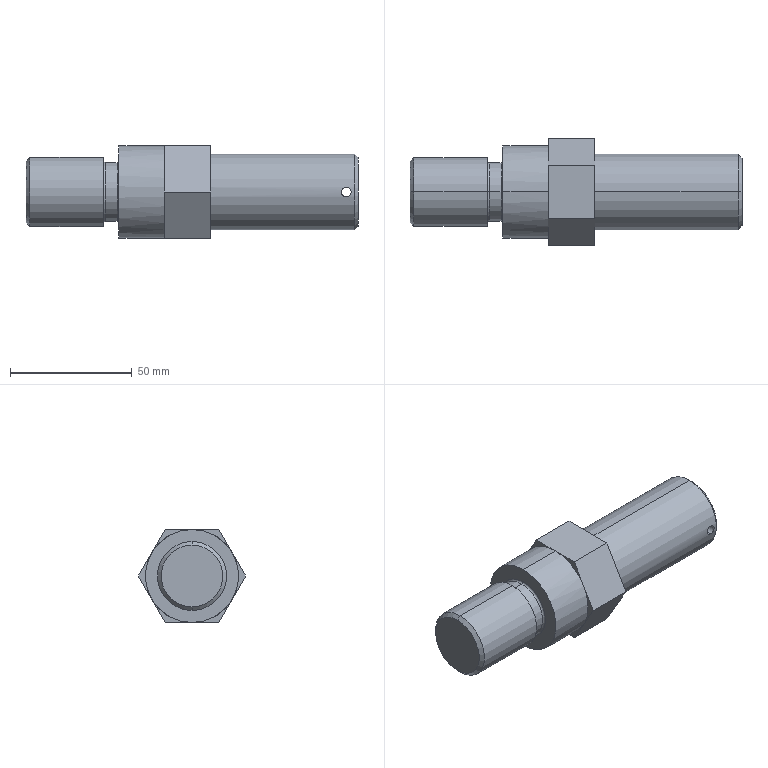Part | SolidWorks | features ICE 2, Chamfer 1, Fillet 1, Revolution 1 | 1 solid | 35 faces | box 136.144 x 43.994 x 38.1 mm | volume 113370 mm3 | plane 17 | cylinder 10 | torus 4 | cone 4 | commonest cylinder face diameters 3.969 x2 24.13 x2 28.321 x2 31.115 x2 38.1 x2
STEP:
#1=CARTESIAN_POINT('',(131.318,-15.43,-1.984));
#2=VERTEX_POINT('',#1);
#3=CARTESIAN_POINT('',(131.318,-15.43,1.984));
#4=VERTEX_POINT('',#3);
#5=CARTESIAN_POINT('',(131.318,-15.43,-1.984));
#6=CARTESIAN_POINT('',(131.059,-15.43,-1.984));
#7=CARTESIAN_POINT('',(130.798,-15.437,-1.932));
#8=CARTESIAN_POINT('',(130.32,-15.461,-1.734));
#9=CARTESIAN_POINT('',(130.099,-15.477,-1.587));
#10=CARTESIAN_POINT('',(129.824,-15.502,-1.313));
#11=CARTESIAN_POINT('',(129.74,-15.511,-1.211));
#12=CARTESIAN_POINT('',(129.596,-15.526,-0.9954));
#13=CARTESIAN_POINT('',(129.535,-15.533,-0.8815));
#14=CARTESIAN_POINT('',(129.436,-15.545,-0.6413));
#15=CARTESIAN_POINT('',(129.397,-15.549,-0.5153));
#16=CARTESIAN_POINT('',(129.347,-15.556,-0.2617));
#17=CARTESIAN_POINT('',(129.334,-15.557,-0.1326));
#18=CARTESIAN_POINT('',(129.334,-15.558,0.1298));
#19=CARTESIAN_POINT('',(129.346,-15.556,0.2588));
#20=CARTESIAN_POINT('',(129.397,-15.55,0.5126));
#21=CARTESIAN_POINT('',(129.435,-15.545,0.6388));
#22=CARTESIAN_POINT('',(129.534,-15.533,0.879));
#23=CARTESIAN_POINT('',(129.595,-15.526,0.993));
#24=CARTESIAN_POINT('',(129.739,-15.511,1.209));
#25=CARTESIAN_POINT('',(129.823,-15.502,1.311));
#26=CARTESIAN_POINT('',(130.097,-15.478,1.585));
#27=CARTESIAN_POINT('',(130.318,-15.461,1.733));
#28=CARTESIAN_POINT('',(130.795,-15.437,1.932));
#29=CARTESIAN_POINT('',(131.056,-15.43,1.984));
#30=CARTESIAN_POINT('',(131.318,-15.43,1.984));
#31=B_SPLINE_CURVE_WITH_KNOTS('',3,(#5,#6,#7,#8,#9,#10,#11,#12,#13,#14,#15,#16,#17,#18,#19,#20,#21,#22,#23,#24,#25,#26,#27,#28,#29,#30),.UNSPECIFIED.,.F.,.F.,(4,2,2,2,2,2,2,2,2,2,2,2,4),(0.00621,0.006986,0.007763,0.008151,0.008539,0.008927,0.009315,0.009703,0.01009,0.01048,0.01087,0.01164,0.01242),.UNSPECIFIED.);
#32=EDGE_CURVE('',#2,#4,#31,.T.);
#33=ORIENTED_EDGE('',*,*,#32,.F.);
#34=CARTESIAN_POINT('',(131.318,15.43,-1.984));
#35=VERTEX_POINT('',#34);
#36=CARTESIAN_POINT('',(131.318,-25.,-1.984));
#37=DIRECTION('',(0.,1.,0.));
#38=VECTOR('',#37,1000.);
#39=LINE('',#36,#38);
#40=EDGE_CURVE('',#2,#35,#39,.T.);
#41=ORIENTED_EDGE('',*,*,#40,.T.);
#42=CARTESIAN_POINT('',(131.318,15.43,1.984));
#43=VERTEX_POINT('',#42);
#44=CARTESIAN_POINT('',(131.318,15.43,1.984));
#45=CARTESIAN_POINT('',(131.187,15.43,1.984));
#46=CARTESIAN_POINT('',(131.058,15.432,1.971));
#47=CARTESIAN_POINT('',(130.804,15.438,1.921));
#48=CARTESIAN_POINT('',(130.678,15.443,1.883));
#49=CARTESIAN_POINT('',(130.438,15.455,1.783));
#50=CARTESIAN_POINT('',(130.324,15.462,1.722));
#51=CARTESIAN_POINT('',(130.108,15.477,1.578));
#52=CARTESIAN_POINT('',(130.006,15.486,1.494));
#53=CARTESIAN_POINT('',(129.732,15.511,1.22));
#54=CARTESIAN_POINT('',(129.584,15.527,0.9987));
#55=CARTESIAN_POINT('',(129.386,15.551,0.5212));
#56=CARTESIAN_POINT('',(129.334,15.557,0.2599));
#57=CARTESIAN_POINT('',(129.334,15.558,-0.1288));
#58=CARTESIAN_POINT('',(129.347,15.556,-0.2605));
#59=CARTESIAN_POINT('',(129.397,15.549,-0.5151));
#60=CARTESIAN_POINT('',(129.435,15.545,-0.6389));
#61=CARTESIAN_POINT('',(129.534,15.533,-0.8793));
#62=CARTESIAN_POINT('',(129.596,15.526,-0.9953));
#63=CARTESIAN_POINT('',(129.74,15.511,-1.21));
#64=CARTESIAN_POINT('',(129.822,15.502,-1.31));
#65=CARTESIAN_POINT('',(130.007,15.486,-1.496));
#66=CARTESIAN_POINT('',(130.107,15.477,-1.578));
#67=CARTESIAN_POINT('',(130.322,15.462,-1.721));
#68=CARTESIAN_POINT('',(130.438,15.455,-1.783));
#69=CARTESIAN_POINT('',(130.679,15.443,-1.883));
#70=CARTESIAN_POINT('',(130.802,15.439,-1.921));
#71=CARTESIAN_POINT('',(131.057,15.432,-1.971));
#72=CARTESIAN_POINT('',(131.188,15.43,-1.984));
#73=CARTESIAN_POINT('',(131.318,15.43,-1.984));
#74=B_SPLINE_CURVE_WITH_KNOTS('',3,(#44,#45,#46,#47,#48,#49,#50,#51,#52,#53,#54,#55,#56,#57,#58,#59,#60,#61,#62,#63,#64,#65,#66,#67,#68,#69,#70,#71,#72,#73),.UNSPECIFIED.,.F.,.F.,(4,2,2,2,2,2,2,2,2,2,2,2,2,2,4),(0.,0.0003881,0.0007763,0.001164,0.001553,0.002329,0.003105,0.003493,0.003881,0.00427,0.004658,0.005046,0.005434,0.005822,0.00621),.UNSPECIFIED.);
#75=EDGE_CURVE('',#43,#35,#74,.T.);
#76=ORIENTED_EDGE('',*,*,#75,.F.);
#77=CARTESIAN_POINT('',(131.318,-25.,1.984));
#78=DIRECTION('',(0.,1.,0.));
#79=VECTOR('',#78,1000.);
#80=LINE('',#77,#79);
#81=EDGE_CURVE('',#4,#43,#80,.T.);
#82=ORIENTED_EDGE('',*,*,#81,.F.);
#83=EDGE_LOOP('',(#33,#41,#76,#82));
#84=FACE_OUTER_BOUND('',#83,.T.);
#85=CARTESIAN_POINT('',(131.318,-25.,0.));
#86=DIRECTION('',(0.,1.,0.));
#87=DIRECTION('',(0.,0.,1.));
#88=AXIS2_PLACEMENT_3D('',#85,#86,#87);
#89=CYLINDRICAL_SURFACE('',#88,1.984);
#90=ADVANCED_FACE('',(#84),#89,.F.);
#91=CARTESIAN_POINT('',(38.1,0.,12.827));
#92=VERTEX_POINT('',#91);
#93=CARTESIAN_POINT('',(38.1,0.,-12.827));
#94=VERTEX_POINT('',#93);
#95=CARTESIAN_POINT('',(38.1,0.,0.));
#96=DIRECTION('',(1.,0.,0.));
#97=DIRECTION('',(0.,0.,-1.));
#98=AXIS2_PLACEMENT_3D('',#95,#96,#97);
#99=CIRCLE('',#98,12.827);
#100=EDGE_CURVE('',#92,#94,#99,.T.);
#101=ORIENTED_EDGE('',*,*,#100,.F.);
#102=CARTESIAN_POINT('',(37.338,0.,12.065));
#103=VERTEX_POINT('',#102);
#104=CARTESIAN_POINT('',(37.338,0.,12.827));
#105=DIRECTION('',(0.,1.,0.));
#106=DIRECTION('',(0.,0.,1.));
#107=AXIS2_PLACEMENT_3D('',#104,#105,#106);
#108=CIRCLE('',#107,0.762);
#109=EDGE_CURVE('',#92,#103,#108,.T.);
#110=ORIENTED_EDGE('',*,*,#109,.T.);
#111=CARTESIAN_POINT('',(37.338,0.,-12.065));
#112=VERTEX_POINT('',#111);
#113=CARTESIAN_POINT('',(37.338,0.,0.));
#114=DIRECTION('',(-1.,0.,0.));
#115=DIRECTION('',(0.,0.,-1.));
#116=AXIS2_PLACEMENT_3D('',#113,#114,#115);
#117=CIRCLE('',#116,12.065);
#118=EDGE_CURVE('',#112,#103,#117,.T.);
#119=ORIENTED_EDGE('',*,*,#118,.F.);
#120=CARTESIAN_POINT('',(37.338,0.,-12.827));
#121=DIRECTION('',(0.,-1.,0.));
#122=DIRECTION('',(0.,0.,-1.));
#123=AXIS2_PLACEMENT_3D('',#120,#121,#122);
#124=CIRCLE('',#123,0.762);
#125=EDGE_CURVE('',#94,#112,#124,.T.);
#126=ORIENTED_EDGE('',*,*,#125,.F.);
#127=EDGE_LOOP('',(#101,#110,#119,#126));
#128=FACE_OUTER_BOUND('',#127,.T.);
#129=CARTESIAN_POINT('',(37.338,0.,0.));
#130=DIRECTION('',(1.,0.,0.));
#131=DIRECTION('',(0.,0.,-1.));
#132=AXIS2_PLACEMENT_3D('',#129,#130,#131);
#133=TOROIDAL_SURFACE('',#132,12.827,0.762);
#134=ADVANCED_FACE('',(#128),#133,.F.);
#135=CARTESIAN_POINT('',(31.75,0.,-12.827));
#136=VERTEX_POINT('',#135);
#137=CARTESIAN_POINT('',(31.75,0.,12.827));
#138=VERTEX_POINT('',#137);
#139=CARTESIAN_POINT('',(31.75,0.,0.));
#140=DIRECTION('',(-1.,0.,0.));
#141=DIRECTION('',(0.,0.,1.));
#142=AXIS2_PLACEMENT_3D('',#139,#140,#141);
#143=CIRCLE('',#142,12.827);
#144=EDGE_CURVE('',#136,#138,#143,.T.);
#145=ORIENTED_EDGE('',*,*,#144,.F.);
#146=CARTESIAN_POINT('',(32.512,0.,-12.065));
#147=VERTEX_POINT('',#146);
#148=CARTESIAN_POINT('',(32.512,0.,-12.827));
#149=DIRECTION('',(0.,1.,0.));
#150=DIRECTION('',(0.,0.,1.));
#151=AXIS2_PLACEMENT_3D('',#148,#149,#150);
#152=CIRCLE('',#151,0.762);
#153=EDGE_CURVE('',#136,#147,#152,.T.);
#154=ORIENTED_EDGE('',*,*,#153,.T.);
#155=CARTESIAN_POINT('',(32.512,0.,12.065));
#156=VERTEX_POINT('',#155);
#157=CARTESIAN_POINT('',(32.512,0.,0.));
#158=DIRECTION('',(1.,0.,0.));
#159=DIRECTION('',(0.,0.,1.));
#160=AXIS2_PLACEMENT_3D('',#157,#158,#159);
#161=CIRCLE('',#160,12.065);
#162=EDGE_CURVE('',#156,#147,#161,.T.);
#163=ORIENTED_EDGE('',*,*,#162,.F.);
#164=CARTESIAN_POINT('',(32.512,0.,12.827));
#165=DIRECTION('',(0.,-1.,0.));
#166=DIRECTION('',(0.,0.,-1.));
#167=AXIS2_PLACEMENT_3D('',#164,#165,#166);
#168=CIRCLE('',#167,0.762);
#169=EDGE_CURVE('',#138,#156,#168,.T.);
#170=ORIENTED_EDGE('',*,*,#169,.F.);
#171=EDGE_LOOP('',(#145,#154,#163,#170));
#172=FACE_OUTER_BOUND('',#171,.T.);
#173=CARTESIAN_POINT('',(32.512,0.,0.));
#174=DIRECTION('',(-1.,0.,0.));
#175=DIRECTION('',(0.,0.,1.));
#176=AXIS2_PLACEMENT_3D('',#173,#174,#175);
#177=TOROIDAL_SURFACE('',#176,12.827,0.762);
#178=ADVANCED_FACE('',(#172),#177,.F.);
#179=ORIENTED_EDGE('',*,*,#75,.T.);
#180=CARTESIAN_POINT('',(131.318,15.43,-1.984));
#181=CARTESIAN_POINT('',(131.577,15.43,-1.984));
#182=CARTESIAN_POINT('',(131.838,15.437,-1.932));
#183=CARTESIAN_POINT('',(132.316,15.461,-1.734));
#184=CARTESIAN_POINT('',(132.537,15.477,-1.587));
#185=CARTESIAN_POINT('',(132.812,15.502,-1.313));
#186=CARTESIAN_POINT('',(132.896,15.511,-1.211));
#187=CARTESIAN_POINT('',(133.04,15.526,-0.9954));
#188=CARTESIAN_POINT('',(133.101,15.533,-0.8815));
#189=CARTESIAN_POINT('',(133.2,15.545,-0.6413));
#190=CARTESIAN_POINT('',(133.239,15.549,-0.5153));
#191=CARTESIAN_POINT('',(133.289,15.556,-0.2617));
#192=CARTESIAN_POINT('',(133.302,15.557,-0.1326));
#193=CARTESIAN_POINT('',(133.302,15.558,0.1298));
#194=CARTESIAN_POINT('',(133.29,15.556,0.2588));
#195=CARTESIAN_POINT('',(133.239,15.55,0.5126));
#196=CARTESIAN_POINT('',(133.201,15.545,0.6388));
#197=CARTESIAN_POINT('',(133.102,15.533,0.879));
#198=CARTESIAN_POINT('',(133.041,15.526,0.993));
#199=CARTESIAN_POINT('',(132.897,15.511,1.209));
#200=CARTESIAN_POINT('',(132.813,15.502,1.311));
#201=CARTESIAN_POINT('',(132.539,15.478,1.585));
#202=CARTESIAN_POINT('',(132.318,15.461,1.733));
#203=CARTESIAN_POINT('',(131.841,15.437,1.932));
#204=CARTESIAN_POINT('',(131.58,15.43,1.984));
#205=CARTESIAN_POINT('',(131.318,15.43,1.984));
#206=B_SPLINE_CURVE_WITH_KNOTS('',3,(#180,#181,#182,#183,#184,#185,#186,#187,#188,#189,#190,#191,#192,#193,#194,#195,#196,#197,#198,#199,#200,#201,#202,#203,#204,#205),.UNSPECIFIED.,.F.,.F.,(4,2,2,2,2,2,2,2,2,2,2,2,4),(0.00621,0.006986,0.007763,0.008151,0.008539,0.008927,0.009315,0.009703,0.01009,0.01048,0.01087,0.01164,0.01242),.UNSPECIFIED.);
#207=EDGE_CURVE('',#35,#43,#206,.T.);
#208=ORIENTED_EDGE('',*,*,#207,.T.);
#209=EDGE_LOOP('',(#179,#208));
#210=FACE_BOUND('',#209,.T.);
#211=CARTESIAN_POINT('',(134.62,0.,15.557));
#212=VERTEX_POINT('',#211);
#213=CARTESIAN_POINT('',(134.62,0.,-15.557));
#214=VERTEX_POINT('',#213);
#215=CARTESIAN_POINT('',(134.62,0.,0.));
#216=DIRECTION('',(-1.,0.,0.));
#217=DIRECTION('',(0.,0.,1.));
#218=AXIS2_PLACEMENT_3D('',#215,#216,#217);
#219=CIRCLE('',#218,15.557);
#220=EDGE_CURVE('',#212,#214,#219,.T.);
#221=ORIENTED_EDGE('',*,*,#220,.T.);
#222=CARTESIAN_POINT('',(75.692,0.,-15.557));
#223=VERTEX_POINT('',#222);
#224=CARTESIAN_POINT('',(0.,0.,-15.557));
#225=DIRECTION('',(-1.,0.,0.));
#226=VECTOR('',#225,1000.);
#227=LINE('',#224,#226);
#228=EDGE_CURVE('',#214,#223,#227,.T.);
#229=ORIENTED_EDGE('',*,*,#228,.T.);
#230=CARTESIAN_POINT('',(75.692,0.,15.557));
#231=VERTEX_POINT('',#230);
#232=CARTESIAN_POINT('',(75.692,0.,0.));
#233=DIRECTION('',(-1.,0.,0.));
#234=DIRECTION('',(0.,0.,1.));
#235=AXIS2_PLACEMENT_3D('',#232,#233,#234);
#236=CIRCLE('',#235,15.557);
#237=EDGE_CURVE('',#231,#223,#236,.T.);
#238=ORIENTED_EDGE('',*,*,#237,.F.);
#239=CARTESIAN_POINT('',(0.,0.,15.557));
#240=DIRECTION('',(-1.,0.,0.));
#241=VECTOR('',#240,1000.);
#242=LINE('',#239,#241);
#243=EDGE_CURVE('',#212,#231,#242,.T.);
#244=ORIENTED_EDGE('',*,*,#243,.F.);
#245=EDGE_LOOP('',(#221,#229,#238,#244));
#246=FACE_OUTER_BOUND('',#245,.T.);
#247=CARTESIAN_POINT('',(0.,0.,0.));
#248=DIRECTION('',(-1.,0.,0.));
#249=DIRECTION('',(0.,0.,1.));
#250=AXIS2_PLACEMENT_3D('',#247,#248,#249);
#251=CYLINDRICAL_SURFACE('',#250,15.557);
#252=ADVANCED_FACE('',(#210,#246),#251,.T.);
#253=CARTESIAN_POINT('',(136.144,0.,-14.034));
#254=VERTEX_POINT('',#253);
#255=CARTESIAN_POINT('',(136.144,0.,14.034));
#256=VERTEX_POINT('',#255);
#257=CARTESIAN_POINT('',(136.144,0.,0.));
#258=DIRECTION('',(1.,0.,0.));
#259=DIRECTION('',(0.,0.,1.));
#260=AXIS2_PLACEMENT_3D('',#257,#258,#259);
#261=CIRCLE('',#260,14.034);
#262=EDGE_CURVE('',#254,#256,#261,.T.);
#263=ORIENTED_EDGE('',*,*,#262,.F.);
#264=CARTESIAN_POINT('',(134.62,0.,-15.557));
#265=DIRECTION('',(-0.7071,0.,-0.7071));
#266=VECTOR('',#265,1000.);
#267=LINE('',#264,#266);
#268=EDGE_CURVE('',#254,#214,#267,.T.);
#269=ORIENTED_EDGE('',*,*,#268,.T.);
#270=ORIENTED_EDGE('',*,*,#220,.F.);
#271=CARTESIAN_POINT('',(134.62,0.,15.557));
#272=DIRECTION('',(-0.7071,0.,0.7071));
#273=VECTOR('',#272,1000.);
#274=LINE('',#271,#273);
#275=EDGE_CURVE('',#256,#212,#274,.T.);
#276=ORIENTED_EDGE('',*,*,#275,.F.);
#277=EDGE_LOOP('',(#263,#269,#270,#276));
#278=FACE_OUTER_BOUND('',#277,.T.);
#279=CARTESIAN_POINT('',(134.62,0.,0.));
#280=DIRECTION('',(-1.,0.,0.));
#281=DIRECTION('',(0.,0.,1.));
#282=AXIS2_PLACEMENT_3D('',#279,#280,#281);
#283=CONICAL_SURFACE('',#282,15.557,0.7854);
#284=ADVANCED_FACE('',(#278),#283,.T.);
#285=CARTESIAN_POINT('',(0.,0.,12.636));
#286=VERTEX_POINT('',#285);
#287=CARTESIAN_POINT('',(0.,0.,-12.636));
#288=VERTEX_POINT('',#287);
#289=CARTESIAN_POINT('',(0.,0.,0.));
#290=DIRECTION('',(-1.,0.,0.));
#291=DIRECTION('',(0.,0.,-1.));
#292=AXIS2_PLACEMENT_3D('',#289,#290,#291);
#293=CIRCLE('',#292,12.636);
#294=EDGE_CURVE('',#286,#288,#293,.T.);
#295=ORIENTED_EDGE('',*,*,#294,.F.);
#296=CARTESIAN_POINT('',(1.524,0.,14.161));
#297=VERTEX_POINT('',#296);
#298=CARTESIAN_POINT('',(0.,0.,12.636));
#299=DIRECTION('',(0.7071,0.,0.7071));
#300=VECTOR('',#299,1000.);
#301=LINE('',#298,#300);
#302=EDGE_CURVE('',#286,#297,#301,.T.);
#303=ORIENTED_EDGE('',*,*,#302,.T.);
#304=CARTESIAN_POINT('',(1.524,0.,-14.161));
#305=VERTEX_POINT('',#304);
#306=CARTESIAN_POINT('',(1.524,0.,0.));
#307=DIRECTION('',(1.,0.,0.));
#308=DIRECTION('',(0.,0.,-1.));
#309=AXIS2_PLACEMENT_3D('',#306,#307,#308);
#310=CIRCLE('',#309,14.161);
#311=EDGE_CURVE('',#305,#297,#310,.T.);
#312=ORIENTED_EDGE('',*,*,#311,.F.);
#313=CARTESIAN_POINT('',(0.,0.,-12.636));
#314=DIRECTION('',(0.7071,0.,-0.7071));
#315=VECTOR('',#314,1000.);
#316=LINE('',#313,#315);
#317=EDGE_CURVE('',#288,#305,#316,.T.);
#318=ORIENTED_EDGE('',*,*,#317,.F.);
#319=EDGE_LOOP('',(#295,#303,#312,#318));
#320=FACE_OUTER_BOUND('',#319,.T.);
#321=CARTESIAN_POINT('',(0.,0.,0.));
#322=DIRECTION('',(1.,0.,0.));
#323=DIRECTION('',(0.,0.,-1.));
#324=AXIS2_PLACEMENT_3D('',#321,#322,#323);
#325=CONICAL_SURFACE('',#324,12.636,0.7854);
#326=ADVANCED_FACE('',(#320),#325,.T.);
#327=CARTESIAN_POINT('',(37.338,0.,0.));
#328=DIRECTION('',(-1.,0.,0.));
#329=DIRECTION('',(0.,0.,-1.));
#330=AXIS2_PLACEMENT_3D('',#327,#328,#329);
#331=CIRCLE('',#330,12.065);
#332=EDGE_CURVE('',#103,#112,#331,.T.);
#333=ORIENTED_EDGE('',*,*,#332,.T.);
#334=CARTESIAN_POINT('',(0.,0.,-12.065));
#335=DIRECTION('',(-1.,0.,0.));
#336=VECTOR('',#335,1000.);
#337=LINE('',#334,#336);
#338=EDGE_CURVE('',#112,#147,#337,.T.);
#339=ORIENTED_EDGE('',*,*,#338,.T.);
#340=CARTESIAN_POINT('',(32.512,0.,0.));
#341=DIRECTION('',(1.,0.,0.));
#342=DIRECTION('',(0.,0.,1.));
#343=AXIS2_PLACEMENT_3D('',#340,#341,#342);
#344=CIRCLE('',#343,12.065);
#345=EDGE_CURVE('',#147,#156,#344,.T.);
#346=ORIENTED_EDGE('',*,*,#345,.T.);
#347=CARTESIAN_POINT('',(0.,0.,12.065));
#348=DIRECTION('',(-1.,0.,0.));
#349=VECTOR('',#348,1000.);
#350=LINE('',#347,#349);
#351=EDGE_CURVE('',#103,#156,#350,.T.);
#352=ORIENTED_EDGE('',*,*,#351,.F.);
#353=EDGE_LOOP('',(#333,#339,#346,#352));
#354=FACE_OUTER_BOUND('',#353,.T.);
#355=CARTESIAN_POINT('',(0.,0.,0.));
#356=DIRECTION('',(-1.,0.,0.));
#357=DIRECTION('',(0.,0.,1.));
#358=AXIS2_PLACEMENT_3D('',#355,#356,#357);
#359=CYLINDRICAL_SURFACE('',#358,12.065);
#360=ADVANCED_FACE('',(#354),#359,.T.);
#361=CARTESIAN_POINT('',(31.75,0.,14.161));
#362=VERTEX_POINT('',#361);
#363=CARTESIAN_POINT('',(31.75,0.,-14.161));
#364=VERTEX_POINT('',#363);
#365=CARTESIAN_POINT('',(31.75,0.,0.));
#366=DIRECTION('',(-1.,0.,0.));
#367=DIRECTION('',(0.,0.,1.));
#368=AXIS2_PLACEMENT_3D('',#365,#366,#367);
#369=CIRCLE('',#368,14.161);
#370=EDGE_CURVE('',#362,#364,#369,.T.);
#371=ORIENTED_EDGE('',*,*,#370,.T.);
#372=CARTESIAN_POINT('',(0.,0.,-14.161));
#373=DIRECTION('',(-1.,0.,0.));
#374=VECTOR('',#373,1000.);
#375=LINE('',#372,#374);
#376=EDGE_CURVE('',#364,#305,#375,.T.);
#377=ORIENTED_EDGE('',*,*,#376,.T.);
#378=ORIENTED_EDGE('',*,*,#311,.T.);
#379=CARTESIAN_POINT('',(0.,0.,14.161));
#380=DIRECTION('',(-1.,0.,0.));
#381=VECTOR('',#380,1000.);
#382=LINE('',#379,#381);
#383=EDGE_CURVE('',#362,#297,#382,.T.);
#384=ORIENTED_EDGE('',*,*,#383,.F.);
#385=EDGE_LOOP('',(#371,#377,#378,#384));
#386=FACE_OUTER_BOUND('',#385,.T.);
#387=CARTESIAN_POINT('',(0.,0.,0.));
#388=DIRECTION('',(-1.,0.,0.));
#389=DIRECTION('',(0.,0.,1.));
#390=AXIS2_PLACEMENT_3D('',#387,#388,#389);
#391=CYLINDRICAL_SURFACE('',#390,14.161);
#392=ADVANCED_FACE('',(#386),#391,.T.);
#393=CARTESIAN_POINT('',(56.769,0.,-19.05));
#394=VERTEX_POINT('',#393);
#395=CARTESIAN_POINT('',(56.769,16.498,-9.525));
#396=VERTEX_POINT('',#395);
#397=CARTESIAN_POINT('',(56.769,0.,0.));
#398=DIRECTION('',(1.,0.,0.));
#399=DIRECTION('',(0.,0.,-1.));
#400=AXIS2_PLACEMENT_3D('',#397,#398,#399);
#401=CIRCLE('',#400,19.05);
#402=EDGE_CURVE('',#394,#396,#401,.T.);
#403=ORIENTED_EDGE('',*,*,#402,.F.);
#404=CARTESIAN_POINT('',(38.1,0.,-19.05));
#405=VERTEX_POINT('',#404);
#406=CARTESIAN_POINT('',(0.,0.,-19.05));
#407=DIRECTION('',(-1.,0.,0.));
#408=VECTOR('',#407,1000.);
#409=LINE('',#406,#408);
#410=EDGE_CURVE('',#394,#405,#409,.T.);
#411=ORIENTED_EDGE('',*,*,#410,.T.);
#412=CARTESIAN_POINT('',(38.1,0.,19.05));
#413=VERTEX_POINT('',#412);
#414=CARTESIAN_POINT('',(38.1,0.,0.));
#415=DIRECTION('',(-1.,0.,0.));
#416=DIRECTION('',(0.,0.,1.));
#417=AXIS2_PLACEMENT_3D('',#414,#415,#416);
#418=CIRCLE('',#417,19.05);
#419=EDGE_CURVE('',#413,#405,#418,.T.);
#420=ORIENTED_EDGE('',*,*,#419,.F.);
#421=CARTESIAN_POINT('',(56.769,0.,19.05));
#422=VERTEX_POINT('',#421);
#423=CARTESIAN_POINT('',(0.,0.,19.05));
#424=DIRECTION('',(-1.,0.,0.));
#425=VECTOR('',#424,1000.);
#426=LINE('',#423,#425);
#427=EDGE_CURVE('',#422,#413,#426,.T.);
#428=ORIENTED_EDGE('',*,*,#427,.F.);
#429=CARTESIAN_POINT('',(56.769,16.498,9.525));
#430=VERTEX_POINT('',#429);
#431=CARTESIAN_POINT('',(56.769,0.,0.));
#432=DIRECTION('',(1.,0.,0.));
#433=DIRECTION('',(0.,0.,-1.));
#434=AXIS2_PLACEMENT_3D('',#431,#432,#433);
#435=CIRCLE('',#434,19.05);
#436=EDGE_CURVE('',#430,#422,#435,.T.);
#437=ORIENTED_EDGE('',*,*,#436,.F.);
#438=CARTESIAN_POINT('',(56.769,0.,0.));
#439=DIRECTION('',(1.,0.,0.));
#440=DIRECTION('',(0.,0.,-1.));
#441=AXIS2_PLACEMENT_3D('',#438,#439,#440);
#442=CIRCLE('',#441,19.05);
#443=EDGE_CURVE('',#396,#430,#442,.T.);
#444=ORIENTED_EDGE('',*,*,#443,.F.);
#445=EDGE_LOOP('',(#403,#411,#420,#428,#437,#444));
#446=FACE_OUTER_BOUND('',#445,.T.);
#447=CARTESIAN_POINT('',(0.,0.,0.));
#448=DIRECTION('',(-1.,0.,0.));
#449=DIRECTION('',(0.,0.,1.));
#450=AXIS2_PLACEMENT_3D('',#447,#448,#449);
#451=CYLINDRICAL_SURFACE('',#450,19.05);
#452=ADVANCED_FACE('',(#446),#451,.T.);
#453=ORIENTED_EDGE('',*,*,#410,.F.);
#454=CARTESIAN_POINT('',(56.769,-16.498,-9.525));
#455=VERTEX_POINT('',#454);
#456=CARTESIAN_POINT('',(56.769,0.,0.));
#457=DIRECTION('',(1.,0.,0.));
#458=DIRECTION('',(0.,0.,-1.));
#459=AXIS2_PLACEMENT_3D('',#456,#457,#458);
#460=CIRCLE('',#459,19.05);
#461=EDGE_CURVE('',#455,#394,#460,.T.);
#462=ORIENTED_EDGE('',*,*,#461,.F.);
#463=CARTESIAN_POINT('',(56.769,-16.498,9.525));
#464=VERTEX_POINT('',#463);
#465=CARTESIAN_POINT('',(56.769,0.,0.));
#466=DIRECTION('',(1.,0.,0.));
#467=DIRECTION('',(0.,0.,-1.));
#468=AXIS2_PLACEMENT_3D('',#465,#466,#467);
#469=CIRCLE('',#468,19.05);
#470=EDGE_CURVE('',#464,#455,#469,.T.);
#471=ORIENTED_EDGE('',*,*,#470,.F.);
#472=CARTESIAN_POINT('',(56.769,0.,0.));
#473=DIRECTION('',(1.,0.,0.));
#474=DIRECTION('',(0.,0.,-1.));
#475=AXIS2_PLACEMENT_3D('',#472,#473,#474);
#476=CIRCLE('',#475,19.05);
#477=EDGE_CURVE('',#422,#464,#476,.T.);
#478=ORIENTED_EDGE('',*,*,#477,.F.);
#479=ORIENTED_EDGE('',*,*,#427,.T.);
#480=CARTESIAN_POINT('',(38.1,0.,0.));
#481=DIRECTION('',(-1.,0.,0.));
#482=DIRECTION('',(0.,0.,1.));
#483=AXIS2_PLACEMENT_3D('',#480,#481,#482);
#484=CIRCLE('',#483,19.05);
#485=EDGE_CURVE('',#405,#413,#484,.T.);
#486=ORIENTED_EDGE('',*,*,#485,.F.);
#487=EDGE_LOOP('',(#453,#462,#471,#478,#479,#486));
#488=FACE_OUTER_BOUND('',#487,.T.);
#489=CARTESIAN_POINT('',(0.,0.,0.));
#490=DIRECTION('',(-1.,0.,0.));
#491=DIRECTION('',(0.,0.,1.));
#492=AXIS2_PLACEMENT_3D('',#489,#490,#491);
#493=CYLINDRICAL_SURFACE('',#492,19.05);
#494=ADVANCED_FACE('',(#488),#493,.T.);
#495=CARTESIAN_POINT('',(0.,0.,0.));
#496=DIRECTION('',(-1.,0.,0.));
#497=DIRECTION('',(0.,0.,-1.));
#498=AXIS2_PLACEMENT_3D('',#495,#496,#497);
#499=CIRCLE('',#498,12.636);
#500=EDGE_CURVE('',#288,#286,#499,.T.);
#501=ORIENTED_EDGE('',*,*,#500,.T.);
#502=ORIENTED_EDGE('',*,*,#294,.T.);
#503=EDGE_LOOP('',(#501,#502));
#504=FACE_OUTER_BOUND('',#503,.T.);
#505=CARTESIAN_POINT('',(0.,0.,0.));
#506=DIRECTION('',(1.,0.,0.));
#507=DIRECTION('',(0.,0.,-1.));
#508=AXIS2_PLACEMENT_3D('',#505,#506,#507);
#509=PLANE('',#508);
#510=ADVANCED_FACE('',(#504),#509,.F.);
#511=ORIENTED_EDGE('',*,*,#376,.F.);
#512=CARTESIAN_POINT('',(31.75,0.,0.));
#513=DIRECTION('',(-1.,0.,0.));
#514=DIRECTION('',(0.,0.,1.));
#515=AXIS2_PLACEMENT_3D('',#512,#513,#514);
#516=CIRCLE('',#515,14.161);
#517=EDGE_CURVE('',#364,#362,#516,.T.);
#518=ORIENTED_EDGE('',*,*,#517,.T.);
#519=ORIENTED_EDGE('',*,*,#383,.T.);
#520=CARTESIAN_POINT('',(1.524,0.,0.));
#521=DIRECTION('',(1.,0.,0.));
#522=DIRECTION('',(0.,0.,-1.));
#523=AXIS2_PLACEMENT_3D('',#520,#521,#522);
#524=CIRCLE('',#523,14.161);
#525=EDGE_CURVE('',#297,#305,#524,.T.);
#526=ORIENTED_EDGE('',*,*,#525,.T.);
#527=EDGE_LOOP('',(#511,#518,#519,#526));
#528=FACE_OUTER_BOUND('',#527,.T.);
#529=CARTESIAN_POINT('',(0.,0.,0.));
#530=DIRECTION('',(-1.,0.,0.));
#531=DIRECTION('',(0.,0.,1.));
#532=AXIS2_PLACEMENT_3D('',#529,#530,#531);
#533=CYLINDRICAL_SURFACE('',#532,14.161);
#534=ADVANCED_FACE('',(#528),#533,.T.);
#535=CARTESIAN_POINT('',(31.75,0.,0.));
#536=DIRECTION('',(-1.,0.,0.));
#537=DIRECTION('',(0.,0.,1.));
#538=AXIS2_PLACEMENT_3D('',#535,#536,#537);
#539=CIRCLE('',#538,12.827);
#540=EDGE_CURVE('',#138,#136,#539,.T.);
#541=ORIENTED_EDGE('',*,*,#540,.T.);
#542=ORIENTED_EDGE('',*,*,#144,.T.);
#543=EDGE_LOOP('',(#541,#542));
#544=FACE_BOUND('',#543,.T.);
#545=ORIENTED_EDGE('',*,*,#370,.F.);
#546=ORIENTED_EDGE('',*,*,#517,.F.);
#547=EDGE_LOOP('',(#545,#546));
#548=FACE_OUTER_BOUND('',#547,.T.);
#549=CARTESIAN_POINT('',(31.75,14.161,0.));
#550=DIRECTION('',(-1.,0.,0.));
#551=DIRECTION('',(0.,0.,1.));
#552=AXIS2_PLACEMENT_3D('',#549,#550,#551);
#553=PLANE('',#552);
#554=ADVANCED_FACE('',(#544,#548),#553,.F.);
#555=ORIENTED_EDGE('',*,*,#338,.F.);
#556=ORIENTED_EDGE('',*,*,#118,.T.);
#557=ORIENTED_EDGE('',*,*,#351,.T.);
#558=ORIENTED_EDGE('',*,*,#162,.T.);
#559=EDGE_LOOP('',(#555,#556,#557,#558));
#560=FACE_OUTER_BOUND('',#559,.T.);
#561=CARTESIAN_POINT('',(0.,0.,0.));
#562=DIRECTION('',(-1.,0.,0.));
#563=DIRECTION('',(0.,0.,1.));
#564=AXIS2_PLACEMENT_3D('',#561,#562,#563);
#565=CYLINDRICAL_SURFACE('',#564,12.065);
#566=ADVANCED_FACE('',(#560),#565,.T.);
#567=CARTESIAN_POINT('',(38.1,0.,0.));
#568=DIRECTION('',(1.,0.,0.));
#569=DIRECTION('',(0.,0.,-1.));
#570=AXIS2_PLACEMENT_3D('',#567,#568,#569);
#571=CIRCLE('',#570,12.827);
#572=EDGE_CURVE('',#94,#92,#571,.T.);
#573=ORIENTED_EDGE('',*,*,#572,.T.);
#574=ORIENTED_EDGE('',*,*,#100,.T.);
#575=EDGE_LOOP('',(#573,#574));
#576=FACE_BOUND('',#575,.T.);
#577=ORIENTED_EDGE('',*,*,#419,.T.);
#578=ORIENTED_EDGE('',*,*,#485,.T.);
#579=EDGE_LOOP('',(#577,#578));
#580=FACE_OUTER_BOUND('',#579,.T.);
#581=CARTESIAN_POINT('',(38.1,12.065,0.));
#582=DIRECTION('',(1.,0.,0.));
#583=DIRECTION('',(0.,0.,-1.));
#584=AXIS2_PLACEMENT_3D('',#581,#582,#583);
#585=PLANE('',#584);
#586=ADVANCED_FACE('',(#576,#580),#585,.F.);
#587=ORIENTED_EDGE('',*,*,#302,.F.);
#588=ORIENTED_EDGE('',*,*,#500,.F.);
#589=ORIENTED_EDGE('',*,*,#317,.T.);
#590=ORIENTED_EDGE('',*,*,#525,.F.);
#591=EDGE_LOOP('',(#587,#588,#589,#590));
#592=FACE_OUTER_BOUND('',#591,.T.);
#593=CARTESIAN_POINT('',(0.,0.,0.));
#594=DIRECTION('',(1.,0.,0.));
#595=DIRECTION('',(0.,0.,-1.));
#596=AXIS2_PLACEMENT_3D('',#593,#594,#595);
#597=CONICAL_SURFACE('',#596,12.636,0.7854);
#598=ADVANCED_FACE('',(#592),#597,.T.);
#599=CARTESIAN_POINT('',(56.769,10.999,-19.05));
#600=VERTEX_POINT('',#599);
#601=CARTESIAN_POINT('',(56.769,-10.999,-19.05));
#602=DIRECTION('',(0.,1.,0.));
#603=VECTOR('',#602,1000.);
#604=LINE('',#601,#603);
#605=EDGE_CURVE('',#394,#600,#604,.T.);
#606=ORIENTED_EDGE('',*,*,#605,.F.);
#607=ORIENTED_EDGE('',*,*,#402,.T.);
#608=CARTESIAN_POINT('',(56.769,10.999,-19.05));
#609=DIRECTION('',(0.,0.5,0.866));
#610=VECTOR('',#609,1000.);
#611=LINE('',#608,#610);
#612=EDGE_CURVE('',#600,#396,#611,.T.);
#613=ORIENTED_EDGE('',*,*,#612,.F.);
#614=EDGE_LOOP('',(#606,#607,#613));
#615=FACE_OUTER_BOUND('',#614,.T.);
#616=CARTESIAN_POINT('',(56.769,0.,0.));
#617=DIRECTION('',(1.,0.,0.));
#618=DIRECTION('',(0.,0.,-1.));
#619=AXIS2_PLACEMENT_3D('',#616,#617,#618);
#620=PLANE('',#619);
#621=ADVANCED_FACE('',(#615),#620,.F.);
#622=CARTESIAN_POINT('',(56.769,21.997,0.));
#623=VERTEX_POINT('',#622);
#624=CARTESIAN_POINT('',(56.769,10.999,-19.05));
#625=DIRECTION('',(0.,0.5,0.866));
#626=VECTOR('',#625,1000.);
#627=LINE('',#624,#626);
#628=EDGE_CURVE('',#396,#623,#627,.T.);
#629=ORIENTED_EDGE('',*,*,#628,.F.);
#630=ORIENTED_EDGE('',*,*,#443,.T.);
#631=CARTESIAN_POINT('',(56.769,21.997,0.));
#632=DIRECTION('',(0.,-0.5,0.866));
#633=VECTOR('',#632,1000.);
#634=LINE('',#631,#633);
#635=EDGE_CURVE('',#623,#430,#634,.T.);
#636=ORIENTED_EDGE('',*,*,#635,.F.);
#637=EDGE_LOOP('',(#629,#630,#636));
#638=FACE_OUTER_BOUND('',#637,.T.);
#639=CARTESIAN_POINT('',(56.769,0.,0.));
#640=DIRECTION('',(1.,0.,0.));
#641=DIRECTION('',(0.,0.,-1.));
#642=AXIS2_PLACEMENT_3D('',#639,#640,#641);
#643=PLANE('',#642);
#644=ADVANCED_FACE('',(#638),#643,.F.);
#645=CARTESIAN_POINT('',(56.769,10.999,19.05));
#646=VERTEX_POINT('',#645);
#647=CARTESIAN_POINT('',(56.769,21.997,0.));
#648=DIRECTION('',(0.,-0.5,0.866));
#649=VECTOR('',#648,1000.);
#650=LINE('',#647,#649);
#651=EDGE_CURVE('',#430,#646,#650,.T.);
#652=ORIENTED_EDGE('',*,*,#651,.F.);
#653=ORIENTED_EDGE('',*,*,#436,.T.);
#654=CARTESIAN_POINT('',(56.769,10.999,19.05));
#655=DIRECTION('',(0.,-1.,0.));
#656=VECTOR('',#655,1000.);
#657=LINE('',#654,#656);
#658=EDGE_CURVE('',#646,#422,#657,.T.);
#659=ORIENTED_EDGE('',*,*,#658,.F.);
#660=EDGE_LOOP('',(#652,#653,#659));
#661=FACE_OUTER_BOUND('',#660,.T.);
#662=CARTESIAN_POINT('',(56.769,0.,0.));
#663=DIRECTION('',(1.,0.,0.));
#664=DIRECTION('',(0.,0.,-1.));
#665=AXIS2_PLACEMENT_3D('',#662,#663,#664);
#666=PLANE('',#665);
#667=ADVANCED_FACE('',(#661),#666,.F.);
#668=CARTESIAN_POINT('',(56.769,-10.999,19.05));
#669=VERTEX_POINT('',#668);
#670=CARTESIAN_POINT('',(56.769,10.999,19.05));
#671=DIRECTION('',(0.,-1.,0.));
#672=VECTOR('',#671,1000.);
#673=LINE('',#670,#672);
#674=EDGE_CURVE('',#422,#669,#673,.T.);
#675=ORIENTED_EDGE('',*,*,#674,.F.);
#676=ORIENTED_EDGE('',*,*,#477,.T.);
#677=CARTESIAN_POINT('',(56.769,-10.999,19.05));
#678=DIRECTION('',(0.,-0.5,-0.866));
#679=VECTOR('',#678,1000.);
#680=LINE('',#677,#679);
#681=EDGE_CURVE('',#669,#464,#680,.T.);
#682=ORIENTED_EDGE('',*,*,#681,.F.);
#683=EDGE_LOOP('',(#675,#676,#682));
#684=FACE_OUTER_BOUND('',#683,.T.);
#685=CARTESIAN_POINT('',(56.769,0.,0.));
#686=DIRECTION('',(1.,0.,0.));
#687=DIRECTION('',(0.,0.,-1.));
#688=AXIS2_PLACEMENT_3D('',#685,#686,#687);
#689=PLANE('',#688);
#690=ADVANCED_FACE('',(#684),#689,.F.);
#691=CARTESIAN_POINT('',(56.769,-21.997,0.));
#692=VERTEX_POINT('',#691);
#693=CARTESIAN_POINT('',(56.769,-10.999,19.05));
#694=DIRECTION('',(0.,-0.5,-0.866));
#695=VECTOR('',#694,1000.);
#696=LINE('',#693,#695);
#697=EDGE_CURVE('',#464,#692,#696,.T.);
#698=ORIENTED_EDGE('',*,*,#697,.F.);
#699=ORIENTED_EDGE('',*,*,#470,.T.);
#700=CARTESIAN_POINT('',(56.769,-21.997,0.));
#701=DIRECTION('',(0.,0.5,-0.866));
#702=VECTOR('',#701,1000.);
#703=LINE('',#700,#702);
#704=EDGE_CURVE('',#692,#455,#703,.T.);
#705=ORIENTED_EDGE('',*,*,#704,.F.);
#706=EDGE_LOOP('',(#698,#699,#705));
#707=FACE_OUTER_BOUND('',#706,.T.);
#708=CARTESIAN_POINT('',(56.769,0.,0.));
#709=DIRECTION('',(1.,0.,0.));
#710=DIRECTION('',(0.,0.,-1.));
#711=AXIS2_PLACEMENT_3D('',#708,#709,#710);
#712=PLANE('',#711);
#713=ADVANCED_FACE('',(#707),#712,.F.);
#714=CARTESIAN_POINT('',(56.769,-10.999,-19.05));
#715=VERTEX_POINT('',#714);
#716=CARTESIAN_POINT('',(56.769,-21.997,0.));
#717=DIRECTION('',(0.,0.5,-0.866));
#718=VECTOR('',#717,1000.);
#719=LINE('',#716,#718);
#720=EDGE_CURVE('',#455,#715,#719,.T.);
#721=ORIENTED_EDGE('',*,*,#720,.F.);
#722=ORIENTED_EDGE('',*,*,#461,.T.);
#723=CARTESIAN_POINT('',(56.769,-10.999,-19.05));
#724=DIRECTION('',(0.,1.,0.));
#725=VECTOR('',#724,1000.);
#726=LINE('',#723,#725);
#727=EDGE_CURVE('',#715,#394,#726,.T.);
#728=ORIENTED_EDGE('',*,*,#727,.F.);
#729=EDGE_LOOP('',(#721,#722,#728));
#730=FACE_OUTER_BOUND('',#729,.T.);
#731=CARTESIAN_POINT('',(56.769,0.,0.));
#732=DIRECTION('',(1.,0.,0.));
#733=DIRECTION('',(0.,0.,-1.));
#734=AXIS2_PLACEMENT_3D('',#731,#732,#733);
#735=PLANE('',#734);
#736=ADVANCED_FACE('',(#730),#735,.F.);
#737=ORIENTED_EDGE('',*,*,#612,.T.);
#738=ORIENTED_EDGE('',*,*,#628,.T.);
#739=CARTESIAN_POINT('',(75.692,21.997,0.));
#740=VERTEX_POINT('',#739);
#741=CARTESIAN_POINT('',(56.769,21.997,0.));
#742=DIRECTION('',(1.,0.,0.));
#743=VECTOR('',#742,1000.);
#744=LINE('',#741,#743);
#745=EDGE_CURVE('',#623,#740,#744,.T.);
#746=ORIENTED_EDGE('',*,*,#745,.T.);
#747=CARTESIAN_POINT('',(75.692,10.999,-19.05));
#748=VERTEX_POINT('',#747);
#749=CARTESIAN_POINT('',(75.692,10.999,-19.05));
#750=DIRECTION('',(0.,0.5,0.866));
#751=VECTOR('',#750,1000.);
#752=LINE('',#749,#751);
#753=EDGE_CURVE('',#748,#740,#752,.T.);
#754=ORIENTED_EDGE('',*,*,#753,.F.);
#755=CARTESIAN_POINT('',(56.769,10.999,-19.05));
#756=DIRECTION('',(1.,0.,0.));
#757=VECTOR('',#756,1000.);
#758=LINE('',#755,#757);
#759=EDGE_CURVE('',#600,#748,#758,.T.);
#760=ORIENTED_EDGE('',*,*,#759,.F.);
#761=EDGE_LOOP('',(#737,#738,#746,#754,#760));
#762=FACE_OUTER_BOUND('',#761,.T.);
#763=CARTESIAN_POINT('',(56.769,10.999,-19.05));
#764=DIRECTION('',(0.,0.866,-0.5));
#765=DIRECTION('',(0.,0.5,0.866));
#766=AXIS2_PLACEMENT_3D('',#763,#764,#765);
#767=PLANE('',#766);
#768=ADVANCED_FACE('',(#762),#767,.T.);
#769=ORIENTED_EDGE('',*,*,#727,.T.);
#770=ORIENTED_EDGE('',*,*,#605,.T.);
#771=ORIENTED_EDGE('',*,*,#759,.T.);
#772=CARTESIAN_POINT('',(75.692,-10.999,-19.05));
#773=VERTEX_POINT('',#772);
#774=CARTESIAN_POINT('',(75.692,-10.999,-19.05));
#775=DIRECTION('',(0.,1.,0.));
#776=VECTOR('',#775,1000.);
#777=LINE('',#774,#776);
#778=EDGE_CURVE('',#773,#748,#777,.T.);
#779=ORIENTED_EDGE('',*,*,#778,.F.);
#780=CARTESIAN_POINT('',(56.769,-10.999,-19.05));
#781=DIRECTION('',(1.,0.,0.));
#782=VECTOR('',#781,1000.);
#783=LINE('',#780,#782);
#784=EDGE_CURVE('',#715,#773,#783,.T.);
#785=ORIENTED_EDGE('',*,*,#784,.F.);
#786=EDGE_LOOP('',(#769,#770,#771,#779,#785));
#787=FACE_OUTER_BOUND('',#786,.T.);
#788=CARTESIAN_POINT('',(56.769,-10.999,-19.05));
#789=DIRECTION('',(0.,0.,-1.));
#790=DIRECTION('',(0.,1.,0.));
#791=AXIS2_PLACEMENT_3D('',#788,#789,#790);
#792=PLANE('',#791);
#793=ADVANCED_FACE('',(#787),#792,.T.);
#794=ORIENTED_EDGE('',*,*,#704,.T.);
#795=ORIENTED_EDGE('',*,*,#720,.T.);
#796=ORIENTED_EDGE('',*,*,#784,.T.);
#797=CARTESIAN_POINT('',(75.692,-21.997,0.));
#798=VERTEX_POINT('',#797);
#799=CARTESIAN_POINT('',(75.692,-21.997,0.));
#800=DIRECTION('',(0.,0.5,-0.866));
#801=VECTOR('',#800,1000.);
#802=LINE('',#799,#801);
#803=EDGE_CURVE('',#798,#773,#802,.T.);
#804=ORIENTED_EDGE('',*,*,#803,.F.);
#805=CARTESIAN_POINT('',(56.769,-21.997,0.));
#806=DIRECTION('',(1.,0.,0.));
#807=VECTOR('',#806,1000.);
#808=LINE('',#805,#807);
#809=EDGE_CURVE('',#692,#798,#808,.T.);
#810=ORIENTED_EDGE('',*,*,#809,.F.);
#811=EDGE_LOOP('',(#794,#795,#796,#804,#810));
#812=FACE_OUTER_BOUND('',#811,.T.);
#813=CARTESIAN_POINT('',(56.769,-21.997,0.));
#814=DIRECTION('',(0.,-0.866,-0.5));
#815=DIRECTION('',(0.,0.5,-0.866));
#816=AXIS2_PLACEMENT_3D('',#813,#814,#815);
#817=PLANE('',#816);
#818=ADVANCED_FACE('',(#812),#817,.T.);
#819=ORIENTED_EDGE('',*,*,#681,.T.);
#820=ORIENTED_EDGE('',*,*,#697,.T.);
#821=ORIENTED_EDGE('',*,*,#809,.T.);
#822=CARTESIAN_POINT('',(75.692,-10.999,19.05));
#823=VERTEX_POINT('',#822);
#824=CARTESIAN_POINT('',(75.692,-10.999,19.05));
#825=DIRECTION('',(0.,-0.5,-0.866));
#826=VECTOR('',#825,1000.);
#827=LINE('',#824,#826);
#828=EDGE_CURVE('',#823,#798,#827,.T.);
#829=ORIENTED_EDGE('',*,*,#828,.F.);
#830=CARTESIAN_POINT('',(56.769,-10.999,19.05));
#831=DIRECTION('',(1.,0.,0.));
#832=VECTOR('',#831,1000.);
#833=LINE('',#830,#832);
#834=EDGE_CURVE('',#669,#823,#833,.T.);
#835=ORIENTED_EDGE('',*,*,#834,.F.);
#836=EDGE_LOOP('',(#819,#820,#821,#829,#835));
#837=FACE_OUTER_BOUND('',#836,.T.);
#838=CARTESIAN_POINT('',(56.769,-10.999,19.05));
#839=DIRECTION('',(0.,-0.866,0.5));
#840=DIRECTION('',(0.,-0.5,-0.866));
#841=AXIS2_PLACEMENT_3D('',#838,#839,#840);
#842=PLANE('',#841);
#843=ADVANCED_FACE('',(#837),#842,.T.);
#844=ORIENTED_EDGE('',*,*,#658,.T.);
#845=ORIENTED_EDGE('',*,*,#674,.T.);
#846=ORIENTED_EDGE('',*,*,#834,.T.);
#847=CARTESIAN_POINT('',(75.692,10.999,19.05));
#848=VERTEX_POINT('',#847);
#849=CARTESIAN_POINT('',(75.692,10.999,19.05));
#850=DIRECTION('',(0.,-1.,0.));
#851=VECTOR('',#850,1000.);
#852=LINE('',#849,#851);
#853=EDGE_CURVE('',#848,#823,#852,.T.);
#854=ORIENTED_EDGE('',*,*,#853,.F.);
#855=CARTESIAN_POINT('',(56.769,10.999,19.05));
#856=DIRECTION('',(1.,0.,0.));
#857=VECTOR('',#856,1000.);
#858=LINE('',#855,#857);
#859=EDGE_CURVE('',#646,#848,#858,.T.);
#860=ORIENTED_EDGE('',*,*,#859,.F.);
#861=EDGE_LOOP('',(#844,#845,#846,#854,#860));
#862=FACE_OUTER_BOUND('',#861,.T.);
#863=CARTESIAN_POINT('',(56.769,10.999,19.05));
#864=DIRECTION('',(0.,0.,1.));
#865=DIRECTION('',(0.,-1.,0.));
#866=AXIS2_PLACEMENT_3D('',#863,#864,#865);
#867=PLANE('',#866);
#868=ADVANCED_FACE('',(#862),#867,.T.);
#869=ORIENTED_EDGE('',*,*,#635,.T.);
#870=ORIENTED_EDGE('',*,*,#651,.T.);
#871=ORIENTED_EDGE('',*,*,#859,.T.);
#872=CARTESIAN_POINT('',(75.692,21.997,0.));
#873=DIRECTION('',(0.,-0.5,0.866));
#874=VECTOR('',#873,1000.);
#875=LINE('',#872,#874);
#876=EDGE_CURVE('',#740,#848,#875,.T.);
#877=ORIENTED_EDGE('',*,*,#876,.F.);
#878=ORIENTED_EDGE('',*,*,#745,.F.);
#879=EDGE_LOOP('',(#869,#870,#871,#877,#878));
#880=FACE_OUTER_BOUND('',#879,.T.);
#881=CARTESIAN_POINT('',(56.769,21.997,0.));
#882=DIRECTION('',(0.,0.866,0.5));
#883=DIRECTION('',(0.,-0.5,0.866));
#884=AXIS2_PLACEMENT_3D('',#881,#882,#883);
#885=PLANE('',#884);
#886=ADVANCED_FACE('',(#880),#885,.T.);
#887=CARTESIAN_POINT('',(136.144,0.,0.));
#888=DIRECTION('',(1.,0.,0.));
#889=DIRECTION('',(0.,0.,1.));
#890=AXIS2_PLACEMENT_3D('',#887,#888,#889);
#891=CIRCLE('',#890,14.034);
#892=EDGE_CURVE('',#256,#254,#891,.T.);
#893=ORIENTED_EDGE('',*,*,#892,.T.);
#894=ORIENTED_EDGE('',*,*,#262,.T.);
#895=EDGE_LOOP('',(#893,#894));
#896=FACE_OUTER_BOUND('',#895,.T.);
#897=CARTESIAN_POINT('',(136.144,15.557,0.));
#898=DIRECTION('',(-1.,0.,0.));
#899=DIRECTION('',(0.,0.,1.));
#900=AXIS2_PLACEMENT_3D('',#897,#898,#899);
#901=PLANE('',#900);
#902=ADVANCED_FACE('',(#896),#901,.F.);
#903=ORIENTED_EDGE('',*,*,#268,.F.);
#904=ORIENTED_EDGE('',*,*,#892,.F.);
#905=ORIENTED_EDGE('',*,*,#275,.T.);
#906=CARTESIAN_POINT('',(134.62,0.,0.));
#907=DIRECTION('',(-1.,0.,0.));
#908=DIRECTION('',(0.,0.,1.));
#909=AXIS2_PLACEMENT_3D('',#906,#907,#908);
#910=CIRCLE('',#909,15.557);
#911=EDGE_CURVE('',#214,#212,#910,.T.);
#912=ORIENTED_EDGE('',*,*,#911,.F.);
#913=EDGE_LOOP('',(#903,#904,#905,#912));
#914=FACE_OUTER_BOUND('',#913,.T.);
#915=CARTESIAN_POINT('',(134.62,0.,0.));
#916=DIRECTION('',(-1.,0.,0.));
#917=DIRECTION('',(0.,0.,1.));
#918=AXIS2_PLACEMENT_3D('',#915,#916,#917);
#919=CONICAL_SURFACE('',#918,15.557,0.7854);
#920=ADVANCED_FACE('',(#914),#919,.T.);
#921=ORIENTED_EDGE('',*,*,#228,.F.);
#922=ORIENTED_EDGE('',*,*,#911,.T.);
#923=ORIENTED_EDGE('',*,*,#243,.T.);
#924=CARTESIAN_POINT('',(75.692,0.,0.));
#925=DIRECTION('',(-1.,0.,0.));
#926=DIRECTION('',(0.,0.,1.));
#927=AXIS2_PLACEMENT_3D('',#924,#925,#926);
#928=CIRCLE('',#927,15.557);
#929=EDGE_CURVE('',#223,#231,#928,.T.);
#930=ORIENTED_EDGE('',*,*,#929,.F.);
#931=EDGE_LOOP('',(#921,#922,#923,#930));
#932=FACE_OUTER_BOUND('',#931,.T.);
#933=CARTESIAN_POINT('',(131.318,-15.43,1.984));
#934=CARTESIAN_POINT('',(131.449,-15.43,1.984));
#935=CARTESIAN_POINT('',(131.578,-15.432,1.971));
#936=CARTESIAN_POINT('',(131.832,-15.438,1.921));
#937=CARTESIAN_POINT('',(131.958,-15.443,1.883));
#938=CARTESIAN_POINT('',(132.198,-15.455,1.783));
#939=CARTESIAN_POINT('',(132.312,-15.462,1.722));
#940=CARTESIAN_POINT('',(132.528,-15.477,1.578));
#941=CARTESIAN_POINT('',(132.63,-15.486,1.494));
#942=CARTESIAN_POINT('',(132.904,-15.511,1.22));
#943=CARTESIAN_POINT('',(133.052,-15.527,0.9987));
#944=CARTESIAN_POINT('',(133.25,-15.551,0.5212));
#945=CARTESIAN_POINT('',(133.302,-15.557,0.2599));
#946=CARTESIAN_POINT('',(133.302,-15.558,-0.1288));
#947=CARTESIAN_POINT('',(133.289,-15.556,-0.2605));
#948=CARTESIAN_POINT('',(133.239,-15.549,-0.5151));
#949=CARTESIAN_POINT('',(133.201,-15.545,-0.6389));
#950=CARTESIAN_POINT('',(133.102,-15.533,-0.8793));
#951=CARTESIAN_POINT('',(133.04,-15.526,-0.9953));
#952=CARTESIAN_POINT('',(132.896,-15.511,-1.21));
#953=CARTESIAN_POINT('',(132.814,-15.502,-1.31));
#954=CARTESIAN_POINT('',(132.629,-15.486,-1.496));
#955=CARTESIAN_POINT('',(132.529,-15.477,-1.578));
#956=CARTESIAN_POINT('',(132.314,-15.462,-1.721));
#957=CARTESIAN_POINT('',(132.198,-15.455,-1.783));
#958=CARTESIAN_POINT('',(131.957,-15.443,-1.883));
#959=CARTESIAN_POINT('',(131.834,-15.439,-1.921));
#960=CARTESIAN_POINT('',(131.579,-15.432,-1.971));
#961=CARTESIAN_POINT('',(131.448,-15.43,-1.984));
#962=CARTESIAN_POINT('',(131.318,-15.43,-1.984));
#963=B_SPLINE_CURVE_WITH_KNOTS('',3,(#933,#934,#935,#936,#937,#938,#939,#940,#941,#942,#943,#944,#945,#946,#947,#948,#949,#950,#951,#952,#953,#954,#955,#956,#957,#958,#959,#960,#961,#962),.UNSPECIFIED.,.F.,.F.,(4,2,2,2,2,2,2,2,2,2,2,2,2,2,4),(0.,0.0003881,0.0007763,0.001164,0.001553,0.002329,0.003105,0.003493,0.003881,0.00427,0.004658,0.005046,0.005434,0.005822,0.00621),.UNSPECIFIED.);
#964=EDGE_CURVE('',#4,#2,#963,.T.);
#965=ORIENTED_EDGE('',*,*,#964,.T.);
#966=ORIENTED_EDGE('',*,*,#32,.T.);
#967=EDGE_LOOP('',(#965,#966));
#968=FACE_BOUND('',#967,.T.);
#969=CARTESIAN_POINT('',(0.,0.,0.));
#970=DIRECTION('',(-1.,0.,0.));
#971=DIRECTION('',(0.,0.,1.));
#972=AXIS2_PLACEMENT_3D('',#969,#970,#971);
#973=CYLINDRICAL_SURFACE('',#972,15.557);
#974=ADVANCED_FACE('',(#932,#968),#973,.T.);
#975=ORIENTED_EDGE('',*,*,#803,.T.);
#976=ORIENTED_EDGE('',*,*,#778,.T.);
#977=ORIENTED_EDGE('',*,*,#753,.T.);
#978=ORIENTED_EDGE('',*,*,#876,.T.);
#979=ORIENTED_EDGE('',*,*,#853,.T.);
#980=ORIENTED_EDGE('',*,*,#828,.T.);
#981=EDGE_LOOP('',(#975,#976,#977,#978,#979,#980));
#982=FACE_OUTER_BOUND('',#981,.T.);
#983=ORIENTED_EDGE('',*,*,#237,.T.);
#984=ORIENTED_EDGE('',*,*,#929,.T.);
#985=EDGE_LOOP('',(#983,#984));
#986=FACE_BOUND('',#985,.T.);
#987=CARTESIAN_POINT('',(75.692,19.05,0.));
#988=DIRECTION('',(-1.,0.,0.));
#989=DIRECTION('',(0.,0.,1.));
#990=AXIS2_PLACEMENT_3D('',#987,#988,#989);
#991=PLANE('',#990);
#992=ADVANCED_FACE('',(#982,#986),#991,.F.);
#993=ORIENTED_EDGE('',*,*,#153,.F.);
#994=ORIENTED_EDGE('',*,*,#540,.F.);
#995=ORIENTED_EDGE('',*,*,#169,.T.);
#996=ORIENTED_EDGE('',*,*,#345,.F.);
#997=EDGE_LOOP('',(#993,#994,#995,#996));
#998=FACE_OUTER_BOUND('',#997,.T.);
#999=CARTESIAN_POINT('',(32.512,0.,0.));
#1000=DIRECTION('',(-1.,0.,0.));
#1001=DIRECTION('',(0.,0.,1.));
#1002=AXIS2_PLACEMENT_3D('',#999,#1000,#1001);
#1003=TOROIDAL_SURFACE('',#1002,12.827,0.762);
#1004=ADVANCED_FACE('',(#998),#1003,.F.);
#1005=ORIENTED_EDGE('',*,*,#109,.F.);
#1006=ORIENTED_EDGE('',*,*,#572,.F.);
#1007=ORIENTED_EDGE('',*,*,#125,.T.);
#1008=ORIENTED_EDGE('',*,*,#332,.F.);
#1009=EDGE_LOOP('',(#1005,#1006,#1007,#1008));
#1010=FACE_OUTER_BOUND('',#1009,.T.);
#1011=CARTESIAN_POINT('',(37.338,0.,0.));
#1012=DIRECTION('',(1.,0.,0.));
#1013=DIRECTION('',(0.,0.,-1.));
#1014=AXIS2_PLACEMENT_3D('',#1011,#1012,#1013);
#1015=TOROIDAL_SURFACE('',#1014,12.827,0.762);
#1016=ADVANCED_FACE('',(#1010),#1015,.F.);
#1017=ORIENTED_EDGE('',*,*,#40,.F.);
#1018=ORIENTED_EDGE('',*,*,#964,.F.);
#1019=ORIENTED_EDGE('',*,*,#81,.T.);
#1020=ORIENTED_EDGE('',*,*,#207,.F.);
#1021=EDGE_LOOP('',(#1017,#1018,#1019,#1020));
#1022=FACE_OUTER_BOUND('',#1021,.T.);
#1023=CARTESIAN_POINT('',(131.318,-25.,0.));
#1024=DIRECTION('',(0.,1.,0.));
#1025=DIRECTION('',(0.,0.,1.));
#1026=AXIS2_PLACEMENT_3D('',#1023,#1024,#1025);
#1027=CYLINDRICAL_SURFACE('',#1026,1.984);
#1028=ADVANCED_FACE('',(#1022),#1027,.F.);
#1029=CLOSED_SHELL('',(#90,#134,#178,#252,#284,#326,#360,#392,#452,#494,#510,#534,#554,#566,#586,#598,#621,#644,#667,#690,#713,#736,#768,#793,#818,#843,#868,#886,#902,#920,#974,#992,#1004,#1016,#1028));
#1030=MANIFOLD_SOLID_BREP('',#1029);
#1031=CARTESIAN_POINT('',(0.,0.,0.));
#1032=DIRECTION('',(0.,0.,1.));
#1033=DIRECTION('',(1.,0.,0.));
#1034=AXIS2_PLACEMENT_3D('',#1031,#1032,#1033);
#1035=(LENGTH_UNIT()NAMED_UNIT(*)SI_UNIT(.MILLI.,.METRE.));
#1036=UNCERTAINTY_MEASURE_WITH_UNIT(LENGTH_MEASURE(0.00001),#1035,'','');
#1037=(NAMED_UNIT(*)PLANE_ANGLE_UNIT()SI_UNIT($,.RADIAN.));
#1038=(NAMED_UNIT(*)SI_UNIT($,.STERADIAN.)SOLID_ANGLE_UNIT());
#1039=(GEOMETRIC_REPRESENTATION_CONTEXT(3)GLOBAL_UNCERTAINTY_ASSIGNED_CONTEXT((#1036))GLOBAL_UNIT_ASSIGNED_CONTEXT((#1035,#1037,#1038))REPRESENTATION_CONTEXT('',''));
#1040=ADVANCED_BREP_SHAPE_REPRESENTATION('',(#1030,#1034),#1039);